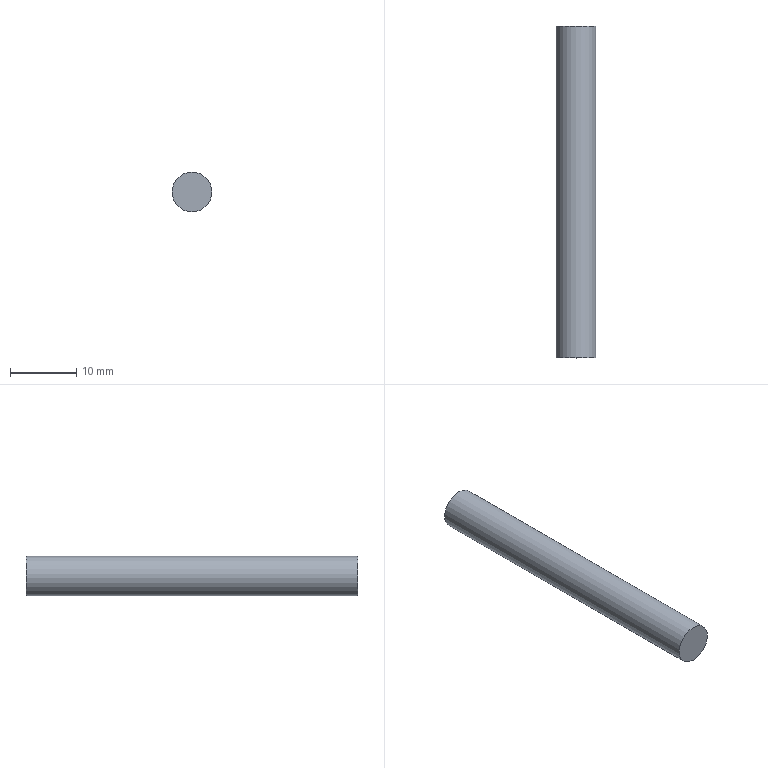Part | STEP file | C_HHSZ50_pin | 1 solid | 3 faces | box 6 x 50 x 6 mm | volume 1414 mm3 | plane 2 | cylinder 1 | commonest cylinder face diameters 6 x1
STEP:
#1=CARTESIAN_POINT('',(0.,25.,3.));
#2=VERTEX_POINT('',#1);
#3=CARTESIAN_POINT('',(0.,25.,0.));
#4=DIRECTION('',(0.,1.,0.));
#5=DIRECTION('',(0.,0.,1.));
#6=AXIS2_PLACEMENT_3D('',#3,#4,#5);
#7=CIRCLE('',#6,3.);
#8=EDGE_CURVE('',#2,#2,#7,.T.);
#9=ORIENTED_EDGE('',*,*,#8,.T.);
#10=EDGE_LOOP('',(#9));
#11=FACE_OUTER_BOUND('',#10,.T.);
#12=CARTESIAN_POINT('',(0.,25.,0.));
#13=DIRECTION('',(0.,-1.,0.));
#14=DIRECTION('',(0.,0.,-1.));
#15=AXIS2_PLACEMENT_3D('',#12,#13,#14);
#16=PLANE('',#15);
#17=ADVANCED_FACE('',(#11),#16,.F.);
#18=ORIENTED_EDGE('',*,*,#8,.F.);
#19=EDGE_LOOP('',(#18));
#20=FACE_OUTER_BOUND('',#19,.T.);
#21=CARTESIAN_POINT('',(0.,-25.,3.));
#22=VERTEX_POINT('',#21);
#23=CARTESIAN_POINT('',(0.,-25.,0.));
#24=DIRECTION('',(0.,1.,0.));
#25=DIRECTION('',(0.,0.,1.));
#26=AXIS2_PLACEMENT_3D('',#23,#24,#25);
#27=CIRCLE('',#26,3.);
#28=EDGE_CURVE('',#22,#22,#27,.T.);
#29=ORIENTED_EDGE('',*,*,#28,.T.);
#30=EDGE_LOOP('',(#29));
#31=FACE_OUTER_BOUND('',#30,.T.);
#32=CARTESIAN_POINT('',(0.,-25.,0.));
#33=DIRECTION('',(0.,1.,0.));
#34=DIRECTION('',(0.,0.,1.));
#35=AXIS2_PLACEMENT_3D('',#32,#33,#34);
#36=CYLINDRICAL_SURFACE('',#35,3.);
#37=ADVANCED_FACE('',(#20,#31),#36,.T.);
#38=ORIENTED_EDGE('',*,*,#28,.F.);
#39=EDGE_LOOP('',(#38));
#40=FACE_OUTER_BOUND('',#39,.T.);
#41=CARTESIAN_POINT('',(0.,-25.,-3.));
#42=DIRECTION('',(0.,1.,0.));
#43=DIRECTION('',(0.,0.,1.));
#44=AXIS2_PLACEMENT_3D('',#41,#42,#43);
#45=PLANE('',#44);
#46=ADVANCED_FACE('',(#40),#45,.F.);
#47=CLOSED_SHELL('',(#17,#37,#46));
#48=MANIFOLD_SOLID_BREP('',#47);
#49=CARTESIAN_POINT('',(0.,0.,0.));
#50=DIRECTION('',(0.,0.,1.));
#51=DIRECTION('',(1.,0.,0.));
#52=AXIS2_PLACEMENT_3D('',#49,#50,#51);
#53=(LENGTH_UNIT()NAMED_UNIT(*)SI_UNIT(.MILLI.,.METRE.));
#54=UNCERTAINTY_MEASURE_WITH_UNIT(LENGTH_MEASURE(0.00001),#53,'','');
#55=(NAMED_UNIT(*)PLANE_ANGLE_UNIT()SI_UNIT($,.RADIAN.));
#56=(NAMED_UNIT(*)SI_UNIT($,.STERADIAN.)SOLID_ANGLE_UNIT());
#57=(GEOMETRIC_REPRESENTATION_CONTEXT(3)GLOBAL_UNCERTAINTY_ASSIGNED_CONTEXT((#54))GLOBAL_UNIT_ASSIGNED_CONTEXT((#53,#55,#56))REPRESENTATION_CONTEXT('',''));
#58=ADVANCED_BREP_SHAPE_REPRESENTATION('',(#48,#52),#57);